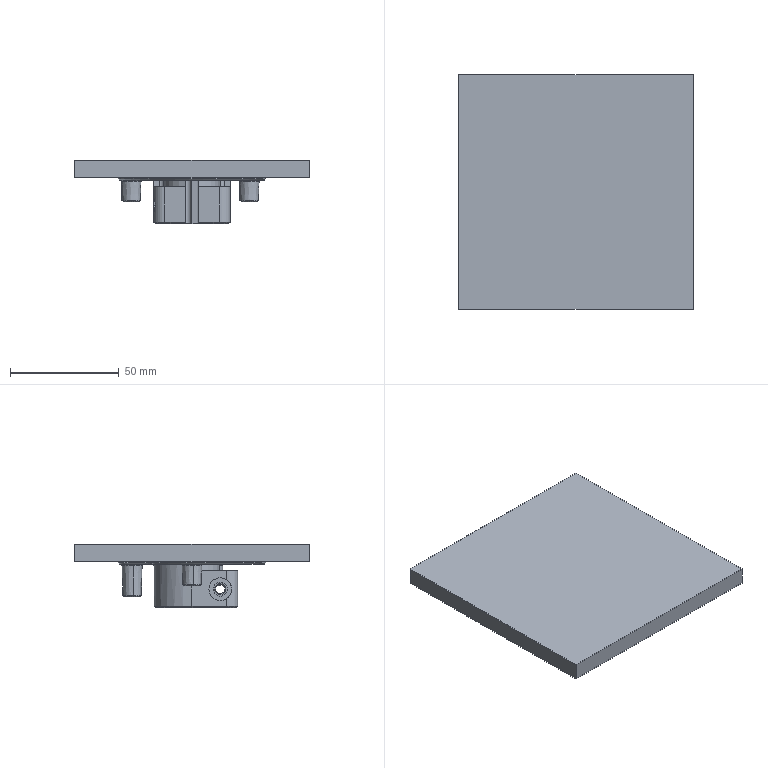NC program | NX | posted with a generic post | part box 108 x 108 x 29 mm
Whole program:
N10 G17 G21 G94 G90
(CAVITY_MILL_COPY_1 , TOOL : D6JING)
N12 T16 M6
N14 G54
N16 G17 G0 G90 X-6.712 Y-4.685 S9500 M3
N18 G43 Z30. H16
N20 Z1.5
N22 G94 G1 X-7.557 Y-4.191 Z1.449 F1000.
N24 X-8.648 Y-3.421 Z1.379
N26 X-8.373 Y-4.116 Z1.34
N28 X-8.272 Y-4.316 Z1.328
N30 X-7.476 Y-5.582 Z1.249
N32 X-6.18 Y-6.99 Z1.149
N34 X-4.625 Y-8.103 Z1.049
N36 X-2.875 Y-8.876 Z0.949
N38 X-1.004 Y-9.276 Z0.848
N40 X-0.257 Y-9.296 Z0.809
N42 X-1.353 Y-8.535 Z0.739
N44 X-3.259 Y-6.951 Z0.609
N46 X-4.208 Y-6.012 Z0.539
N48 X-5.416 Y-5.442 Z0.469
N50 X-7.557 Y-4.191 Z0.339
N52 X-8.648 Y-3.421 Z0.27
N54 X-8.373 Y-4.116 Z0.23
N56 X-8.272 Y-4.316 Z0.219
N58 X-7.476 Y-5.582 Z0.14
N60 X-6.18 Y-6.99 Z0.04
N62 X-4.625 Y-8.103 Z-0.06
N64 X-2.875 Y-8.876 Z-0.161
N66 X-1.004 Y-9.276 Z-0.261
N68 X-0.257 Y-9.296 Z-0.3
N70 G2 X-4.208 Y-6.012 R29.7 F2500.
N72 X-8.648 Y-3.421 R29.7
N74 G3 X-0.257 Y-9.296 R9.3
N76 G1 X1.796 Y-6.339
N78 G2 X-2.11 Y-3.015 R26.1
N80 X-12.018 Y4.689 R26.1
N82 G3 X8.517 Y-9.689 R12.9
N84 G2 X1.796 Y-6.339 R26.1
N86 G1 X3.849 Y-3.382
N88 G2 X0.001 Y-0.001 R22.5
N90 X-11.935 Y11.393 R22.5
N92 G3 X14.788 Y-7.318 R-16.5
N94 G2 X3.849 Y-3.382 R22.5
N96 G1 X5.902 Y-0.424
N98 G2 X2.669 Y2.416 R18.9
N100 G3 X1.358 Y3.334 R3.6
N102 G2 X-10.094 Y17.382 R18.9
N104 G3 X19.786 Y-3.541 R-20.1
N106 G2 X5.902 Y-0.424 R18.9
N108 G1 X7.954 Y2.533
N110 G2 X5.338 Y4.832 R15.3
N112 G3 X2.716 Y6.668 R7.2
N114 G2 X-6.695 Y22.735 R15.3
N116 G3 X23.653 Y1.485 R-23.7
N118 G2 X7.954 Y2.533 R15.3
N120 G1 X10.007 Y5.491
N122 G2 X8.006 Y7.249 R11.7
N124 G3 X4.074 Y10.002 R10.8
N126 G2 X-1.287 Y27.27 R11.7
N128 G3 X26.065 Y8.118 R-27.3
N130 G2 X10.007 Y5.491 R11.7
N132 G1 X12.06 Y8.448
N134 G2 X10.674 Y9.665 R8.1
N136 G3 X5.432 Y13.336 R14.4
N138 G2 X1.852 Y25.484 R8.1
N140 G1 X5.321 Y30.438
N142 G3 X26.783 Y15.411 R-30.9
N144 G1 X23.314 Y10.456
N146 G2 X12.06 Y8.448 R8.1
N148 G3 X11.816 Y8.536 R0.5
N150 G1 Z1.2
N152 G0 X-6.712 Y-4.685
N154 G1 X-7.557 Y-4.191 Z1.149 F1000.
N156 X-8.648 Y-3.421 Z1.079
N158 X-8.373 Y-4.116 Z1.04
N160 X-8.272 Y-4.316 Z1.028
N162 X-7.476 Y-5.582 Z0.949
N164 X-6.18 Y-6.99 Z0.849
N166 X-4.625 Y-8.103 Z0.749
N168 X-2.875 Y-8.876 Z0.649
N170 X-1.004 Y-9.276 Z0.548
N172 X-0.257 Y-9.296 Z0.509
N174 X-1.353 Y-8.535 Z0.439
N176 X-3.259 Y-6.951 Z0.309
N178 X-4.208 Y-6.012 Z0.239
N180 X-5.416 Y-5.442 Z0.169
N182 X-7.557 Y-4.191 Z0.039
N184 X-8.648 Y-3.421 Z-0.03
N186 X-8.373 Y-4.116 Z-0.07
N188 X-8.272 Y-4.316 Z-0.081
N190 X-7.476 Y-5.582 Z-0.16
N192 X-6.18 Y-6.99 Z-0.26
N194 X-4.625 Y-8.103 Z-0.36
N196 X-2.875 Y-8.876 Z-0.461
N198 X-1.004 Y-9.276 Z-0.561
N200 X-0.257 Y-9.296 Z-0.6
N202 G2 X-4.208 Y-6.012 R29.7 F2500.
N204 X-8.648 Y-3.421 R29.7
N206 G3 X-0.257 Y-9.296 R9.3
N208 G1 X1.796 Y-6.339
N210 G2 X-2.11 Y-3.015 R26.1
N212 X-12.018 Y4.689 R26.1
N214 G3 X8.517 Y-9.689 R12.9
N216 G2 X1.796 Y-6.339 R26.1
N218 G1 X3.849 Y-3.382
N220 G2 X0.001 Y-0.001 R22.5
N222 X-11.935 Y11.393 R22.5
N224 G3 X14.788 Y-7.318 R-16.5
N226 G2 X3.849 Y-3.382 R22.5
N228 G1 X5.902 Y-0.424
N230 G2 X2.669 Y2.416 R18.9
N232 G3 X1.358 Y3.334 R3.6
N234 G2 X-10.094 Y17.382 R18.9
N236 G3 X19.786 Y-3.541 R-20.1
N238 G2 X5.902 Y-0.424 R18.9
N240 G1 X7.954 Y2.533
N242 G2 X5.338 Y4.832 R15.3
N244 G3 X2.716 Y6.668 R7.2
N246 G2 X-6.695 Y22.735 R15.3
N248 G3 X23.653 Y1.485 R-23.7
N250 G2 X7.954 Y2.533 R15.3
N252 G1 X10.007 Y5.491
N254 G2 X8.006 Y7.249 R11.7
N256 G3 X4.074 Y10.002 R10.8
N258 G2 X-1.287 Y27.27 R11.7
N260 G3 X26.065 Y8.118 R-27.3
N262 G2 X10.007 Y5.491 R11.7
N264 G1 X12.06 Y8.448
N266 G2 X10.674 Y9.665 R8.1
N268 G3 X5.432 Y13.336 R14.4
N270 G2 X1.852 Y25.484 R8.1
N272 G1 X5.321 Y30.438
N274 G3 X26.783 Y15.411 R-30.9
N276 G1 X23.314 Y10.456
N278 G2 X12.06 Y8.448 R8.1
N280 G3 X11.816 Y8.536 R0.5
N282 G1 Z0.9
N284 G0 X-6.712 Y-4.685
N286 G1 X-7.557 Y-4.191 Z0.849 F1000.
N288 X-8.648 Y-3.421 Z0.779
N290 X-8.373 Y-4.116 Z0.74
N292 X-8.272 Y-4.316 Z0.728
N294 X-7.476 Y-5.582 Z0.649
N296 X-6.18 Y-6.99 Z0.549
N298 X-4.625 Y-8.103 Z0.449
N300 X-2.875 Y-8.876 Z0.349
N302 X-1.004 Y-9.276 Z0.248
N304 X-0.257 Y-9.296 Z0.209
N306 X-1.353 Y-8.535 Z0.139
N308 X-3.259 Y-6.951 Z0.009
N310 X-4.208 Y-6.012 Z-0.061
N312 X-5.416 Y-5.442 Z-0.131
N314 X-7.557 Y-4.191 Z-0.261
N316 X-8.648 Y-3.421 Z-0.33
N318 X-8.373 Y-4.116 Z-0.37
N320 X-8.272 Y-4.316 Z-0.381
N322 X-7.476 Y-5.582 Z-0.46
N324 X-6.18 Y-6.99 Z-0.56
N326 X-4.625 Y-8.103 Z-0.66
N328 X-2.875 Y-8.876 Z-0.761
N330 X-1.004 Y-9.276 Z-0.861
N332 X-0.257 Y-9.296 Z-0.9
N334 G2 X-4.208 Y-6.012 R29.7 F2500.
N336 X-8.648 Y-3.421 R29.7
N338 G3 X-0.257 Y-9.296 R9.3
N340 G1 X1.796 Y-6.339
N342 G2 X-2.11 Y-3.015 R26.1
N344 X-12.018 Y4.689 R26.1
N346 G3 X8.517 Y-9.689 R12.9
N348 G2 X1.796 Y-6.339 R26.1
N350 G1 X3.849 Y-3.382
N352 G2 X0.001 Y-0.001 R22.5
N354 X-11.935 Y11.393 R22.5
N356 G3 X14.788 Y-7.318 R-16.5
N358 G2 X3.849 Y-3.382 R22.5
N360 G1 X5.902 Y-0.424
N362 G2 X2.669 Y2.416 R18.9
N364 G3 X1.358 Y3.334 R3.6
N366 G2 X-10.094 Y17.382 R18.9
N368 G3 X19.786 Y-3.541 R-20.1
N370 G2 X5.902 Y-0.424 R18.9
N372 G1 X7.954 Y2.533
N374 G2 X5.338 Y4.832 R15.3
N376 G3 X2.716 Y6.668 R7.2
N378 G2 X-6.695 Y22.735 R15.3
N380 G3 X23.653 Y1.485 R-23.7
N382 G2 X7.954 Y2.533 R15.3
N384 G1 X10.007 Y5.491
N386 G2 X8.006 Y7.249 R11.7
N388 G3 X4.074 Y10.002 R10.8
N390 G2 X-1.287 Y27.27 R11.7
N392 G3 X26.065 Y8.118 R-27.3
N394 G2 X10.007 Y5.491 R11.7
N396 G1 X12.06 Y8.448
N398 G2 X10.674 Y9.665 R8.1
N400 G3 X5.432 Y13.336 R14.4
N402 G2 X1.852 Y25.484 R8.1
N404 G1 X5.321 Y30.438
N406 G3 X26.783 Y15.411 R-30.9
N408 G1 X23.314 Y10.456
N410 G2 X12.06 Y8.448 R8.1
N412 G3 X11.816 Y8.536 R0.5
N414 G1 Z0.6
N416 G0 X-6.712 Y-4.685
N418 G1 X-7.557 Y-4.191 Z0.549 F1000.
N420 X-8.648 Y-3.421 Z0.479
N422 X-8.373 Y-4.116 Z0.44
N424 X-8.272 Y-4.316 Z0.428
N426 X-7.476 Y-5.582 Z0.349
N428 X-6.18 Y-6.99 Z0.249
N430 X-4.625 Y-8.103 Z0.149
N432 X-2.875 Y-8.876 Z0.049
N434 X-1.004 Y-9.276 Z-0.052
N436 X-0.257 Y-9.296 Z-0.091
N438 X-1.353 Y-8.535 Z-0.161
N440 X-3.259 Y-6.951 Z-0.291
N442 X-4.208 Y-6.012 Z-0.361
N444 X-5.416 Y-5.442 Z-0.431
N446 X-7.557 Y-4.191 Z-0.561
N448 X-8.648 Y-3.421 Z-0.63
N450 X-8.373 Y-4.116 Z-0.67
N452 X-8.272 Y-4.316 Z-0.681
N454 X-7.476 Y-5.582 Z-0.76
N456 X-6.18 Y-6.99 Z-0.86
N458 X-4.625 Y-8.103 Z-0.96
N460 X-2.875 Y-8.876 Z-1.061
N462 X-1.004 Y-9.276 Z-1.161
N464 X-0.257 Y-9.296 Z-1.2
N466 G2 X-4.208 Y-6.012 R29.7 F2500.
N468 X-8.648 Y-3.421 R29.7
N470 G3 X-0.257 Y-9.296 R9.3
N472 G1 X1.796 Y-6.339
N474 G2 X-2.11 Y-3.015 R26.1
N476 X-12.018 Y4.689 R26.1
N478 G3 X8.517 Y-9.689 R12.9
N480 G2 X1.796 Y-6.339 R26.1
N482 G1 X3.849 Y-3.382
N484 G2 X0.001 Y-0.001 R22.5
N486 X-11.935 Y11.393 R22.5
N488 G3 X14.788 Y-7.318 R-16.5
N490 G2 X3.849 Y-3.382 R22.5
N492 G1 X5.902 Y-0.424
N494 G2 X2.669 Y2.416 R18.9
N496 G3 X1.358 Y3.334 R3.6
N498 G2 X-10.094 Y17.382 R18.9
N500 G3 X19.786 Y-3.541 R-20.1
N502 G2 X5.902 Y-0.424 R18.9
N504 G1 X7.954 Y2.533
N506 G2 X5.338 Y4.832 R15.3
N508 G3 X2.716 Y6.668 R7.2
N510 G2 X-6.695 Y22.735 R15.3
N512 G3 X23.653 Y1.485 R-23.7
N514 G2 X7.954 Y2.533 R15.3
N516 G1 X10.007 Y5.491
N518 G2 X8.006 Y7.249 R11.7
N520 G3 X4.074 Y10.002 R10.8
N522 G2 X-1.287 Y27.27 R11.7
N524 G3 X26.065 Y8.118 R-27.3
N526 G2 X10.007 Y5.491 R11.7
N528 G1 X12.06 Y8.448
N530 G2 X10.674 Y9.665 R8.1
N532 G3 X5.432 Y13.336 R14.4
N534 G2 X1.852 Y25.484 R8.1
N536 G1 X5.321 Y30.438
N538 G3 X26.783 Y15.411 R-30.9
N540 G1 X23.314 Y10.456
N542 G2 X12.06 Y8.448 R8.1
N544 G3 X11.816 Y8.536 R0.5
N546 G1 Z0.3
N548 G0 X-6.712 Y-4.685
N550 G1 X-7.557 Y-4.191 Z0.249 F1000.
N552 X-8.648 Y-3.421 Z0.179
N554 X-8.373 Y-4.116 Z0.14
N556 X-8.272 Y-4.316 Z0.128
N558 X-7.476 Y-5.582 Z0.049
N560 X-6.18 Y-6.99 Z-0.051
N562 X-4.625 Y-8.103 Z-0.151
N564 X-2.875 Y-8.876 Z-0.251
N566 X-1.004 Y-9.276 Z-0.352
N568 X-0.257 Y-9.296 Z-0.391
N570 X-1.353 Y-8.535 Z-0.461
N572 X-3.259 Y-6.951 Z-0.591
N574 X-4.208 Y-6.012 Z-0.661
N576 X-5.416 Y-5.442 Z-0.731
N578 X-7.557 Y-4.191 Z-0.861
N580 X-8.648 Y-3.421 Z-0.93
N582 X-8.373 Y-4.116 Z-0.97
N584 X-8.272 Y-4.316 Z-0.981
N586 X-7.476 Y-5.582 Z-1.06
N588 X-6.18 Y-6.99 Z-1.16
N590 X-4.625 Y-8.103 Z-1.26
N592 X-2.875 Y-8.876 Z-1.361
N594 X-1.004 Y-9.276 Z-1.461
N596 X-0.257 Y-9.296 Z-1.5
N598 G2 X-4.208 Y-6.012 R29.7 F2500.
N600 X-8.648 Y-3.421 R29.7
N602 G3 X-0.257 Y-9.296 R9.3
N604 G1 X1.796 Y-6.339
N606 G2 X-2.11 Y-3.015 R26.1
N608 X-12.018 Y4.689 R26.1
N610 G3 X8.517 Y-9.689 R12.9
N612 G2 X1.796 Y-6.339 R26.1
N614 G1 X3.849 Y-3.382
N616 G2 X0.001 Y-0.001 R22.5
N618 X-11.935 Y11.393 R22.5
N620 G3 X14.788 Y-7.318 R-16.5
N622 G2 X3.849 Y-3.382 R22.5
N624 G1 X5.902 Y-0.424
N626 G2 X2.669 Y2.416 R18.9
N628 G3 X1.358 Y3.334 R3.6
N630 G2 X-10.094 Y17.382 R18.9
N632 G3 X19.786 Y-3.541 R-20.1
N634 G2 X5.902 Y-0.424 R18.9
N636 G1 X7.954 Y2.533
N638 G2 X5.338 Y4.832 R15.3
N640 G3 X2.716 Y6.668 R7.2
N642 G2 X-6.695 Y22.735 R15.3
N644 G3 X23.653 Y1.485 R-23.7
N646 G2 X7.954 Y2.533 R15.3
N648 G1 X10.007 Y5.491
N650 G2 X8.006 Y7.249 R11.7
N652 G3 X4.074 Y10.002 R10.8
N654 G2 X-1.287 Y27.27 R11.7
N656 G3 X26.065 Y8.118 R-27.3
N658 G2 X10.007 Y5.491 R11.7
N660 G1 X12.06 Y8.448
N662 G2 X10.674 Y9.665 R8.1
N664 G3 X5.432 Y13.336 R14.4
N666 G2 X1.852 Y25.484 R8.1
N668 G1 X5.321 Y30.438
N670 G3 X26.783 Y15.411 R-30.9
N672 G1 X23.314 Y10.456
N674 G2 X12.06 Y8.448 R8.1
N676 G3 X11.816 Y8.536 R0.5
N678 G1 Z0.
N680 G0 X-6.712 Y-4.685
N682 G1 X-7.557 Y-4.191 Z-0.051 F1000.
N684 X-8.648 Y-3.421 Z-0.121
N686 X-8.373 Y-4.116 Z-0.16
N688 X-8.272 Y-4.316 Z-0.172
N690 X-7.476 Y-5.582 Z-0.251
N692 X-6.18 Y-6.99 Z-0.351
N694 X-4.625 Y-8.103 Z-0.451
N696 X-2.875 Y-8.876 Z-0.551
N698 X-1.004 Y-9.276 Z-0.652
N700 X-0.257 Y-9.296 Z-0.691
N702 X-1.353 Y-8.535 Z-0.761
N704 X-3.259 Y-6.951 Z-0.891
N706 X-4.208 Y-6.012 Z-0.961
N708 X-5.416 Y-5.442 Z-1.031
N710 X-7.557 Y-4.191 Z-1.161
N712 X-8.648 Y-3.421 Z-1.23
N714 X-8.373 Y-4.116 Z-1.27
N716 X-8.272 Y-4.316 Z-1.281
N718 X-7.476 Y-5.582 Z-1.36
N720 X-6.18 Y-6.99 Z-1.46
N722 X-4.625 Y-8.103 Z-1.56
N724 X-2.875 Y-8.876 Z-1.661
N726 X-1.004 Y-9.276 Z-1.761
N728 X-0.257 Y-9.296 Z-1.8
N730 G2 X-4.208 Y-6.012 R29.7 F2500.
N732 X-8.648 Y-3.421 R29.7
N734 G3 X-0.257 Y-9.296 R9.3
N736 G1 X1.796 Y-6.339
N738 G2 X-2.11 Y-3.015 R26.1
N740 X-12.018 Y4.689 R26.1
N742 G3 X8.517 Y-9.689 R12.9
N744 G2 X1.796 Y-6.339 R26.1
N746 G1 X3.849 Y-3.382
N748 G2 X0.001 Y-0.001 R22.5
N750 X-11.935 Y11.393 R22.5
N752 G3 X14.788 Y-7.318 R-16.5
N754 G2 X3.849 Y-3.382 R22.5
N756 G1 X5.902 Y-0.424
N758 G2 X2.669 Y2.416 R18.9
N760 G3 X1.358 Y3.334 R3.6
N762 G2 X-10.094 Y17.382 R18.9
N764 G3 X19.786 Y-3.541 R-20.1
N766 G2 X5.902 Y-0.424 R18.9
N768 G1 X7.954 Y2.533
N770 G2 X5.338 Y4.832 R15.3
N772 G3 X2.716 Y6.668 R7.2
N774 G2 X-6.695 Y22.735 R15.3
N776 G3 X23.653 Y1.485 R-23.7
N778 G2 X7.954 Y2.533 R15.3
N780 G1 X10.007 Y5.491
N782 G2 X8.006 Y7.249 R11.7
N784 G3 X4.074 Y10.002 R10.8
N786 G2 X-1.287 Y27.27 R11.7
N788 G3 X26.065 Y8.118 R-27.3
N790 G2 X10.007 Y5.491 R11.7
N792 G1 X12.06 Y8.448
N794 G2 X10.674 Y9.665 R8.1
N796 G3 X5.432 Y13.336 R14.4
N798 G2 X1.852 Y25.484 R8.1
N800 G1 X5.321 Y30.438
N802 G3 X26.783 Y15.411 R-30.9
N804 G1 X23.314 Y10.456
N806 G2 X12.06 Y8.448 R8.1
N808 G3 X11.816 Y8.536 R0.5
N810 G1 Z-0.3
N812 G0 X-6.712 Y-4.685
N814 G1 X-7.557 Y-4.191 Z-0.351 F1000.
N816 X-8.648 Y-3.421 Z-0.421
N818 X-8.373 Y-4.116 Z-0.46
N820 X-8.272 Y-4.316 Z-0.472
N822 X-7.476 Y-5.582 Z-0.551
N824 X-6.18 Y-6.99 Z-0.651
N826 X-4.625 Y-8.103 Z-0.751
N828 X-2.875 Y-8.876 Z-0.851
N830 X-1.004 Y-9.276 Z-0.952
N832 X-0.257 Y-9.296 Z-0.991
N834 X-1.353 Y-8.535 Z-1.061
N836 X-3.259 Y-6.951 Z-1.191
N838 X-4.208 Y-6.012 Z-1.261
N840 X-5.416 Y-5.442 Z-1.331
N842 X-7.557 Y-4.191 Z-1.461
N844 X-8.648 Y-3.421 Z-1.53
N846 X-8.373 Y-4.116 Z-1.57
N848 X-8.272 Y-4.316 Z-1.581
N850 X-7.476 Y-5.582 Z-1.66
N852 X-6.18 Y-6.99 Z-1.76
N854 X-4.625 Y-8.103 Z-1.86
N856 X-2.875 Y-8.876 Z-1.961
N858 X-1.004 Y-9.276 Z-2.061
N860 X-0.257 Y-9.296 Z-2.1
N862 G2 X-4.208 Y-6.012 R29.7 F2500.
N864 X-8.648 Y-3.421 R29.7
N866 G3 X-0.257 Y-9.296 R9.3
N868 G1 X1.796 Y-6.339
N870 G2 X-2.11 Y-3.015 R26.1
N872 X-12.018 Y4.689 R26.1
N874 G3 X8.517 Y-9.689 R12.9
N876 G2 X1.796 Y-6.339 R26.1
N878 G1 X3.849 Y-3.382
N880 G2 X0.001 Y-0.001 R22.5
N882 X-11.935 Y11.393 R22.5
N884 G3 X14.788 Y-7.318 R-16.5
N886 G2 X3.849 Y-3.382 R22.5
N888 G1 X5.902 Y-0.424
N890 G2 X2.669 Y2.416 R18.9
N892 G3 X1.358 Y3.334 R3.6
N894 G2 X-10.094 Y17.382 R18.9
N896 G3 X19.786 Y-3.541 R-20.1
N898 G2 X5.902 Y-0.424 R18.9
N900 G1 X7.954 Y2.533
N902 G2 X5.338 Y4.832 R15.3
N904 G3 X2.716 Y6.668 R7.2
N906 G2 X-6.695 Y22.735 R15.3
N908 G3 X23.653 Y1.485 R-23.7
N910 G2 X7.954 Y2.533 R15.3
N912 G1 X10.007 Y5.491
N914 G2 X8.006 Y7.249 R11.7
N916 G3 X4.074 Y10.002 R10.8
N918 G2 X-1.287 Y27.27 R11.7
N920 G3 X26.065 Y8.118 R-27.3
N922 G2 X10.007 Y5.491 R11.7
N924 G1 X12.06 Y8.448
N926 G2 X10.674 Y9.665 R8.1
N928 G3 X5.432 Y13.336 R14.4
N930 G2 X1.852 Y25.484 R8.1
N932 G1 X5.321 Y30.438
N934 G3 X26.783 Y15.411 R-30.9
N936 G1 X23.314 Y10.456
N938 G2 X12.06 Y8.448 R8.1
N940 G3 X11.816 Y8.536 R0.5
N942 G1 Z-0.6
N944 G0 X-6.712 Y-4.685
N946 G1 X-7.557 Y-4.191 Z-0.651 F1000.
N948 X-8.648 Y-3.421 Z-0.721
N950 X-8.373 Y-4.116 Z-0.76
N952 X-8.272 Y-4.316 Z-0.772
N954 X-7.476 Y-5.582 Z-0.851
N956 X-6.18 Y-6.99 Z-0.951
N958 X-4.625 Y-8.103 Z-1.051
N960 X-2.875 Y-8.876 Z-1.151
N962 X-1.004 Y-9.276 Z-1.252
N964 X-0.257 Y-9.296 Z-1.291
N966 X-1.353 Y-8.535 Z-1.361
N968 X-3.259 Y-6.951 Z-1.491
N970 X-4.208 Y-6.012 Z-1.561
N972 X-5.416 Y-5.442 Z-1.631
N974 X-7.557 Y-4.191 Z-1.761
N976 X-8.648 Y-3.421 Z-1.83
N978 X-8.373 Y-4.116 Z-1.87
N980 X-8.272 Y-4.316 Z-1.881
N982 X-7.476 Y-5.582 Z-1.96
N984 X-6.18 Y-6.99 Z-2.06
N986 X-4.625 Y-8.103 Z-2.16
N988 X-2.875 Y-8.876 Z-2.261
N990 X-1.004 Y-9.276 Z-2.361
N992 X-0.257 Y-9.296 Z-2.4
N994 G2 X-4.208 Y-6.012 R29.7 F2500.
N996 X-8.648 Y-3.421 R29.7
N998 G3 X-0.257 Y-9.296 R9.3
N1000 G1 X1.796 Y-6.339
N1002 G2 X-2.11 Y-3.015 R26.1
N1004 X-12.018 Y4.689 R26.1
N1006 G3 X8.517 Y-9.689 R12.9
N1008 G2 X1.796 Y-6.339 R26.1
N1010 G1 X3.849 Y-3.382
N1012 G2 X0.001 Y-0.001 R22.5
N1014 X-11.935 Y11.393 R22.5
N1016 G3 X14.788 Y-7.318 R-16.5
N1018 G2 X3.849 Y-3.382 R22.5
N1020 G1 X5.902 Y-0.424
N1022 G2 X2.669 Y2.416 R18.9
N1024 G3 X1.358 Y3.334 R3.6
N1026 G2 X-10.094 Y17.382 R18.9
N1028 G3 X19.786 Y-3.541 R-20.1
N1030 G2 X5.902 Y-0.424 R18.9
N1032 G1 X7.954 Y2.533
N1034 G2 X5.338 Y4.832 R15.3
N1036 G3 X2.716 Y6.668 R7.2
N1038 G2 X-6.695 Y22.735 R15.3
N1040 G3 X23.653 Y1.485 R-23.7
N1042 G2 X7.954 Y2.533 R15.3
N1044 G1 X10.007 Y5.491
N1046 G2 X8.006 Y7.249 R11.7
N1048 G3 X4.074 Y10.002 R10.8
N1050 G2 X-1.287 Y27.27 R11.7
N1052 G3 X26.065 Y8.118 R-27.3
N1054 G2 X10.007 Y5.491 R11.7
N1056 G1 X12.06 Y8.448
N1058 G2 X10.674 Y9.665 R8.1
N1060 G3 X5.432 Y13.336 R14.4
N1062 G2 X1.852 Y25.484 R8.1
N1064 G1 X5.321 Y30.438
N1066 G3 X26.783 Y15.411 R-30.9
N1068 G1 X23.314 Y10.456
N1070 G2 X12.06 Y8.448 R8.1
N1072 G3 X11.816 Y8.536 R0.5
N1074 G1 Z-0.9
N1076 G0 X-6.712 Y-4.685
N1078 G1 X-7.557 Y-4.191 Z-0.951 F1000.
N1080 X-8.648 Y-3.421 Z-1.021
N1082 X-8.373 Y-4.116 Z-1.06
N1084 X-8.272 Y-4.316 Z-1.072
N1086 X-7.476 Y-5.582 Z-1.151
N1088 X-6.18 Y-6.99 Z-1.251
N1090 X-4.625 Y-8.103 Z-1.351
N1092 X-2.875 Y-8.876 Z-1.451
N1094 X-1.004 Y-9.276 Z-1.552
N1096 X-0.257 Y-9.296 Z-1.591
N1098 X-1.353 Y-8.535 Z-1.661
N1100 X-3.259 Y-6.951 Z-1.791
N1102 X-4.208 Y-6.012 Z-1.861
N1104 X-5.416 Y-5.442 Z-1.931
N1106 X-7.557 Y-4.191 Z-2.061
N1108 X-8.648 Y-3.421 Z-2.13
N1110 X-8.373 Y-4.116 Z-2.17
N1112 X-8.272 Y-4.316 Z-2.181
N1114 X-7.476 Y-5.582 Z-2.26
N1116 X-6.18 Y-6.99 Z-2.36
N1118 X-4.625 Y-8.103 Z-2.46
N1120 X-2.875 Y-8.876 Z-2.561
N1122 X-1.004 Y-9.276 Z-2.661
N1124 X-0.257 Y-9.296 Z-2.7
N1126 G2 X-4.208 Y-6.012 R29.7 F2500.
N1128 X-8.648 Y-3.421 R29.7
N1130 G3 X-0.257 Y-9.296 R9.3
N1132 G1 X1.796 Y-6.339
N1134 G2 X-2.11 Y-3.015 R26.1
N1136 X-12.018 Y4.689 R26.1
N1138 G3 X8.517 Y-9.689 R12.9
N1140 G2 X1.796 Y-6.339 R26.1
N1142 G1 X3.849 Y-3.382
N1144 G2 X0.001 Y-0.001 R22.5
N1146 X-11.935 Y11.393 R22.5
N1148 G3 X14.788 Y-7.318 R-16.5
N1150 G2 X3.849 Y-3.382 R22.5
N1152 G1 X5.902 Y-0.424
N1154 G2 X2.669 Y2.416 R18.9
N1156 G3 X1.358 Y3.334 R3.6
N1158 G2 X-10.094 Y17.382 R18.9
N1160 G3 X19.786 Y-3.541 R-20.1
N1162 G2 X5.902 Y-0.424 R18.9
N1164 G1 X7.954 Y2.533
N1166 G2 X5.338 Y4.832 R15.3
N1168 G3 X2.716 Y6.668 R7.2
N1170 G2 X-6.695 Y22.735 R15.3
N1172 G3 X23.653 Y1.485 R-23.7
N1174 G2 X7.954 Y2.533 R15.3
N1176 G1 X10.007 Y5.491
N1178 G2 X8.006 Y7.249 R11.7
N1180 G3 X4.074 Y10.002 R10.8
N1182 G2 X-1.287 Y27.27 R11.7
N1184 G3 X26.065 Y8.118 R-27.3
N1186 G2 X10.007 Y5.491 R11.7
N1188 G1 X12.06 Y8.448
N1190 G2 X10.674 Y9.665 R8.1
N1192 G3 X5.432 Y13.336 R14.4
N1194 G2 X1.852 Y25.484 R8.1
N1196 G1 X5.321 Y30.438
N1198 G3 X26.783 Y15.411 R-30.9
N1200 G1 X23.314 Y10.456
N1202 G2 X12.06 Y8.448 R8.1
N1204 G3 X11.816 Y8.536 R0.5
N1206 G1 Z-1.2
N1208 G0 X-6.712 Y-4.685
N1210 G1 X-7.557 Y-4.191 Z-1.251 F1000.
N1212 X-8.648 Y-3.421 Z-1.321
N1214 X-8.373 Y-4.116 Z-1.36
N1216 X-8.272 Y-4.316 Z-1.372
N1218 X-7.476 Y-5.582 Z-1.451
N1220 X-6.18 Y-6.99 Z-1.551
N1222 X-4.625 Y-8.103 Z-1.651
N1224 X-2.875 Y-8.876 Z-1.751
N1226 X-1.004 Y-9.276 Z-1.852
N1228 X-0.257 Y-9.296 Z-1.891
N1230 X-1.353 Y-8.535 Z-1.961
N1232 X-3.259 Y-6.951 Z-2.091
N1234 X-4.208 Y-6.012 Z-2.161
N1236 X-5.416 Y-5.442 Z-2.231
N1238 X-7.557 Y-4.191 Z-2.361
N1240 X-8.648 Y-3.421 Z-2.43
N1242 X-8.373 Y-4.116 Z-2.47
N1244 X-8.272 Y-4.316 Z-2.481
N1246 X-7.476 Y-5.582 Z-2.56
N1248 X-6.18 Y-6.99 Z-2.66
N1250 X-4.625 Y-8.103 Z-2.76
N1252 X-2.875 Y-8.876 Z-2.861
N1254 X-1.004 Y-9.276 Z-2.961
N1256 X-0.257 Y-9.296 Z-3.
N1258 G2 X-4.208 Y-6.012 R29.7 F2500.
N1260 X-8.648 Y-3.421 R29.7
N1262 G3 X-0.257 Y-9.296 R9.3
N1264 G1 X1.796 Y-6.339
N1266 G2 X-2.11 Y-3.015 R26.1
N1268 X-12.018 Y4.689 R26.1
N1270 G3 X8.517 Y-9.689 R12.9
N1272 G2 X1.796 Y-6.339 R26.1
N1274 G1 X3.849 Y-3.382
N1276 G2 X0.001 Y-0.001 R22.5
N1278 X-11.935 Y11.393 R22.5
N1280 G3 X14.788 Y-7.318 R-16.5
N1282 G2 X3.849 Y-3.382 R22.5
N1284 G1 X5.902 Y-0.424
N1286 G2 X2.669 Y2.416 R18.9
N1288 G3 X1.358 Y3.334 R3.6
N1290 G2 X-10.094 Y17.382 R18.9
N1292 G3 X19.786 Y-3.541 R-20.1
N1294 G2 X5.902 Y-0.424 R18.9
N1296 G1 X7.954 Y2.533
N1298 G2 X5.338 Y4.832 R15.3
N1300 G3 X2.716 Y6.668 R7.2
N1302 G2 X-6.695 Y22.735 R15.3
N1304 G3 X23.653 Y1.485 R-23.7
N1306 G2 X7.954 Y2.533 R15.3
N1308 G1 X10.007 Y5.491
N1310 G2 X8.006 Y7.249 R11.7
N1312 G3 X4.074 Y10.002 R10.8
N1314 G2 X-1.287 Y27.27 R11.7
N1316 G3 X26.065 Y8.118 R-27.3
N1318 G2 X10.007 Y5.491 R11.7
N1320 G1 X12.06 Y8.448
N1322 G2 X10.674 Y9.665 R8.1
N1324 G3 X5.432 Y13.336 R14.4
N1326 G2 X1.852 Y25.484 R8.1
N1328 G1 X5.321 Y30.438
N1330 G3 X26.783 Y15.411 R-30.9
N1332 G1 X23.314 Y10.456
N1334 G2 X12.06 Y8.448 R8.1
N1336 G3 X11.816 Y8.536 R0.5
N1338 G1 Z-1.5
N1340 G0 X-6.712 Y-4.685
N1342 G1 X-7.557 Y-4.191 Z-1.551 F1000.
N1344 X-8.648 Y-3.421 Z-1.621
N1346 X-8.373 Y-4.116 Z-1.66
N1348 X-8.272 Y-4.316 Z-1.672
N1350 X-7.476 Y-5.582 Z-1.751
N1352 X-6.18 Y-6.99 Z-1.851
N1354 X-4.625 Y-8.103 Z-1.951
N1356 X-2.875 Y-8.876 Z-2.051
N1358 X-1.004 Y-9.276 Z-2.152
N1360 X-0.257 Y-9.296 Z-2.191
N1362 X-1.353 Y-8.535 Z-2.261
N1364 X-3.259 Y-6.951 Z-2.391
N1366 X-4.208 Y-6.012 Z-2.461
N1368 X-5.416 Y-5.442 Z-2.531
N1370 X-7.557 Y-4.191 Z-2.661
N1372 X-8.648 Y-3.421 Z-2.73
N1374 X-8.373 Y-4.116 Z-2.77
N1376 X-8.272 Y-4.316 Z-2.781
N1378 X-7.476 Y-5.582 Z-2.86
N1380 X-6.18 Y-6.99 Z-2.96
N1382 X-4.625 Y-8.103 Z-3.06
N1384 X-2.875 Y-8.876 Z-3.161
N1386 X-1.004 Y-9.276 Z-3.261
N1388 X-0.257 Y-9.296 Z-3.3
N1390 G2 X-4.208 Y-6.012 R29.7 F2500.
N1392 X-8.648 Y-3.421 R29.7
N1394 G3 X-0.257 Y-9.296 R9.3
N1396 G1 X1.796 Y-6.339
N1398 G2 X-2.11 Y-3.015 R26.1
N1400 X-12.018 Y4.689 R26.1
N1402 G3 X8.517 Y-9.689 R12.9
N1404 G2 X1.796 Y-6.339 R26.1
N1406 G1 X3.849 Y-3.382
N1408 G2 X0.001 Y-0.001 R22.5
N1410 X-11.935 Y11.393 R22.5
N1412 G3 X14.788 Y-7.318 R-16.5
N1414 G2 X3.849 Y-3.382 R22.5
N1416 G1 X5.902 Y-0.424
N1418 G2 X2.669 Y2.416 R18.9
N1420 G3 X1.358 Y3.334 R3.6
N1422 G2 X-10.094 Y17.382 R18.9
N1424 G3 X19.786 Y-3.541 R-20.1
N1426 G2 X5.902 Y-0.424 R18.9
N1428 G1 X7.954 Y2.533
N1430 G2 X5.338 Y4.832 R15.3
N1432 G3 X2.716 Y6.668 R7.2
N1434 G2 X-6.695 Y22.735 R15.3
N1436 G3 X23.653 Y1.485 R-23.7
N1438 G2 X7.954 Y2.533 R15.3
N1440 G1 X10.007 Y5.491
N1442 G2 X8.006 Y7.249 R11.7
N1444 G3 X4.074 Y10.002 R10.8
N1446 G2 X-1.287 Y27.27 R11.7
N1448 G3 X26.065 Y8.118 R-27.3
N1450 G2 X10.007 Y5.491 R11.7
N1452 G1 X12.06 Y8.448
N1454 G2 X10.674 Y9.665 R8.1
N1456 G3 X5.432 Y13.336 R14.4
N1458 G2 X1.852 Y25.484 R8.1
N1460 G1 X5.321 Y30.438
N1462 G3 X26.783 Y15.411 R-30.9
N1464 G1 X23.314 Y10.456
N1466 G2 X12.06 Y8.448 R8.1
N1468 G3 X11.816 Y8.536 R0.5
N1470 G1 Z-1.8
N1472 G0 X-6.712 Y-4.685
N1474 G1 X-7.557 Y-4.191 Z-1.851 F1000.
N1476 X-8.648 Y-3.421 Z-1.921
N1478 X-8.373 Y-4.116 Z-1.96
N1480 X-8.272 Y-4.316 Z-1.972
N1482 X-7.476 Y-5.582 Z-2.051
N1484 X-6.18 Y-6.99 Z-2.151
N1486 X-4.625 Y-8.103 Z-2.251
N1488 X-2.875 Y-8.876 Z-2.351
N1490 X-1.004 Y-9.276 Z-2.452
N1492 X-0.257 Y-9.296 Z-2.491
N1494 X-1.353 Y-8.535 Z-2.561
N1496 X-3.259 Y-6.951 Z-2.691
N1498 X-4.208 Y-6.012 Z-2.761
N1500 X-5.416 Y-5.442 Z-2.831
N1502 X-7.557 Y-4.191 Z-2.961
N1504 X-8.648 Y-3.421 Z-3.03
N1506 X-8.373 Y-4.116 Z-3.07
N1508 X-8.272 Y-4.316 Z-3.081
N1510 X-7.476 Y-5.582 Z-3.16
N1512 X-6.18 Y-6.99 Z-3.26
N1514 X-4.625 Y-8.103 Z-3.36
N1516 X-2.875 Y-8.876 Z-3.461
N1518 X-1.004 Y-9.276 Z-3.561
N1520 X-0.257 Y-9.296 Z-3.6
N1522 G2 X-4.208 Y-6.012 R29.7 F2500.
N1524 X-8.648 Y-3.421 R29.7
N1526 G3 X-0.257 Y-9.296 R9.3
N1528 G1 X1.796 Y-6.339
N1530 G2 X-2.11 Y-3.015 R26.1
N1532 X-12.018 Y4.689 R26.1
N1534 G3 X8.517 Y-9.689 R12.9
N1536 G2 X1.796 Y-6.339 R26.1
N1538 G1 X3.849 Y-3.382
N1540 G2 X0.001 Y-0.001 R22.5
N1542 X-11.935 Y11.393 R22.5
N1544 G3 X14.788 Y-7.318 R-16.5
N1546 G2 X3.849 Y-3.382 R22.5
N1548 G1 X5.902 Y-0.424
N1550 G2 X2.669 Y2.416 R18.9
N1552 G3 X1.358 Y3.334 R3.6
N1554 G2 X-10.094 Y17.382 R18.9
N1556 G3 X19.786 Y-3.541 R-20.1
N1558 G2 X5.902 Y-0.424 R18.9
N1560 G1 X7.954 Y2.533
N1562 G2 X5.338 Y4.832 R15.3
N1564 G3 X2.716 Y6.668 R7.2
N1566 G2 X-6.695 Y22.735 R15.3
N1568 G3 X23.653 Y1.485 R-23.7
N1570 G2 X7.954 Y2.533 R15.3
N1572 G1 X10.007 Y5.491
N1574 G2 X8.006 Y7.249 R11.7
N1576 G3 X4.074 Y10.002 R10.8
N1578 G2 X-1.287 Y27.27 R11.7
N1580 G3 X26.065 Y8.118 R-27.3
N1582 G2 X10.007 Y5.491 R11.7
N1584 G1 X12.06 Y8.448
N1586 G2 X10.674 Y9.665 R8.1
N1588 G3 X5.432 Y13.336 R14.4
N1590 G2 X1.852 Y25.484 R8.1
N1592 G1 X5.321 Y30.438
N1594 G3 X26.783 Y15.411 R-30.9
N1596 G1 X23.314 Y10.456
N1598 G2 X12.06 Y8.448 R8.1
N1600 G3 X11.816 Y8.536 R0.5
N1602 G1 Z-2.1
N1604 G0 X-6.712 Y-4.685
N1606 G1 X-7.557 Y-4.191 Z-2.151 F1000.
N1608 X-8.648 Y-3.421 Z-2.221
N1610 X-8.373 Y-4.116 Z-2.26
N1612 X-8.272 Y-4.316 Z-2.272
N1614 X-7.476 Y-5.582 Z-2.351
N1616 X-6.18 Y-6.99 Z-2.451
N1618 X-4.625 Y-8.103 Z-2.551
N1620 X-2.875 Y-8.876 Z-2.651
N1622 X-1.004 Y-9.276 Z-2.752
N1624 X-0.257 Y-9.296 Z-2.791
N1626 X-1.353 Y-8.535 Z-2.861
N1628 X-3.259 Y-6.951 Z-2.991
N1630 X-4.208 Y-6.012 Z-3.061
N1632 X-5.416 Y-5.442 Z-3.131
N1634 X-7.557 Y-4.191 Z-3.261
N1636 X-8.648 Y-3.421 Z-3.33
N1638 X-8.373 Y-4.116 Z-3.37
N1640 X-8.272 Y-4.316 Z-3.381
N1642 X-7.476 Y-5.582 Z-3.46
N1644 X-6.18 Y-6.99 Z-3.56
N1646 X-4.625 Y-8.103 Z-3.66
N1648 X-2.875 Y-8.876 Z-3.761
N1650 X-1.004 Y-9.276 Z-3.861
N1652 X-0.257 Y-9.296 Z-3.9
N1654 G2 X-4.208 Y-6.012 R29.7 F2500.
N1656 X-8.648 Y-3.421 R29.7
N1658 G3 X-0.257 Y-9.296 R9.3
N1660 G1 X1.796 Y-6.339
N1662 G2 X-2.11 Y-3.015 R26.1
N1664 X-12.018 Y4.689 R26.1
N1666 G3 X8.517 Y-9.689 R12.9
N1668 G2 X1.796 Y-6.339 R26.1
N1670 G1 X3.849 Y-3.382
N1672 G2 X0.001 Y-0.001 R22.5
N1674 X-11.935 Y11.393 R22.5
N1676 G3 X14.788 Y-7.318 R-16.5
N1678 G2 X3.849 Y-3.382 R22.5
N1680 G1 X5.902 Y-0.424
N1682 G2 X2.669 Y2.416 R18.9
N1684 G3 X1.358 Y3.334 R3.6
N1686 G2 X-10.094 Y17.382 R18.9
N1688 G3 X19.786 Y-3.541 R-20.1
N1690 G2 X5.902 Y-0.424 R18.9
N1692 G1 X7.954 Y2.533
N1694 G2 X5.338 Y4.832 R15.3
N1696 G3 X2.716 Y6.668 R7.2
N1698 G2 X-6.695 Y22.735 R15.3
N1700 G3 X23.653 Y1.485 R-23.7
N1702 G2 X7.954 Y2.533 R15.3
N1704 G1 X10.007 Y5.491
N1706 G2 X8.006 Y7.249 R11.7
N1708 G3 X4.074 Y10.002 R10.8
N1710 G2 X-1.287 Y27.27 R11.7
N1712 G3 X26.065 Y8.118 R-27.3
N1714 G2 X10.007 Y5.491 R11.7
N1716 G1 X12.06 Y8.448
N1718 G2 X10.674 Y9.665 R8.1
N1720 G3 X5.432 Y13.336 R14.4
N1722 G2 X1.852 Y25.484 R8.1
N1724 G1 X5.321 Y30.438
N1726 G3 X26.783 Y15.411 R-30.9
N1728 G1 X23.314 Y10.456
N1730 G2 X12.06 Y8.448 R8.1
N1732 G3 X11.816 Y8.536 R0.5
N1734 G1 Z-2.4
N1736 G0 Z30.
(FLOOR_WALL_1_COPY_1_COPY , TOOL : D6JING)
N1738 X5.248 Y12.801
N1740 Z-2.5
N1742 G1 Z-4. F1000.
N1744 G3 X4.907 Y13.294 R0.6
N1746 X5.337 Y13.105 R8.35 F1200.
N1748 G2 X10.489 Y9.498 R14.15
N1750 G3 X23.518 Y10.313 R8.35
N1752 G1 X26.761 Y14.943
N1754 G2 X4.889 Y30.258 R-30.65
N1756 G1 X1.647 Y25.627
N1758 G3 X4.907 Y13.294 R8.35
N1760 G1 X3.363 Y10.042
N1762 G3 X3.979 Y9.771 R11.95
N1764 G2 X7.82 Y7.081 R10.55
N1766 G3 X25.966 Y7.582 R11.95
N1768 G2 X-1.756 Y26.993 R-27.05
N1770 G3 X3.363 Y10.042 R11.95
N1772 G1 X1.82 Y6.79
N1774 G3 X2.622 Y6.437 R15.55
N1776 G2 X5.152 Y4.665 R6.95
N1778 G3 X23.425 Y1.092 R15.55
N1780 G2 X-6.986 Y22.385 R-23.45
N1782 G3 X1.82 Y6.79 R15.55
N1784 G1 X0.276 Y3.538
N1786 G3 X1.264 Y3.103 R19.15
N1788 G2 X2.483 Y2.249 R3.35
N1790 G3 X19.475 Y-3.843 R19.15
N1792 G2 X-10.272 Y16.986 R-19.85
N1794 G3 X0.276 Y3.538 R19.15
N1796 G1 X-1.268 Y0.285
N1798 G3 X-0.147 Y-0.21 R22.75
N1800 X14.398 Y-7.533 R22.75
N1802 G2 X-12.003 Y10.954 R-16.25
N1804 G3 X-1.268 Y0.285 R22.75
N1806 G1 X-2.811 Y-2.967
N1808 G3 X-2.256 Y-3.222 R26.35
N1810 X8.018 Y-9.784 R26.35
N1812 G2 X-11.936 Y4.189 R12.65
N1814 G3 X-2.811 Y-2.967 R26.35
N1816 G1 X-4.355 Y-6.219
N1818 G3 X-1.128 Y-8.979 R29.95
N1820 G2 X-8.052 Y-4.131 R9.05
N1822 G3 X-4.355 Y-6.219 R29.95
N1824 X-3.757 Y-6.171 R0.6
N1826 G1 Z-2.5
N1828 X1.381 Y27.862 F8000.
N1830 Z-4. F1000.
N1832 X3.106 Y27.711
N1834 G3 X3.65 Y27.965 R0.6
N1836 G1 X5.407 Y30.474 F1200.
N1838 G3 X26.787 Y15.504 R-30.95
N1840 G1 X23.273 Y10.485
N1842 G2 X10.711 Y9.699 R8.05
N1844 G3 X5.451 Y13.383 R14.45
N1846 G2 X1.893 Y25.455 R8.05
N1848 G1 X3.65 Y27.965
N1850 G3 X3.702 Y28.562 R0.6
N1852 G1 X2.719 Y29.251
N1854 Z-2.5
N1856 G0 Z30.
N1858 M5
(11_COPY_1 , TOOL : D6A45)
N1860 T01 M6
N1862 G54
N1864 G17 G0 G90 X2.108 Y24.086 S9500 M3
N1866 G43 Z30. H1
N1868 Z2.
N1870 G94 G1 Z-1. F1000.
N1872 X3.062 Y24.002
N1874 G3 X3.606 Y24.256 R0.6
N1876 G1 X7.165 Y29.339
N1878 G3 X5.855 Y32.519 R2.041
N1880 X28.555 Y16.624 R-33.041
N1882 X25.119 Y16.767 R2.041
N1884 G1 X21.56 Y11.684
N1886 G2 X12.262 Y11.103 R5.959
N1888 G3 X6.239 Y15.32 R16.541
N1890 G2 X3.606 Y24.256 R5.959
N1892 G3 X3.658 Y24.853 R0.6
N1894 G1 X3.219 Y25.795
N1896 Z2.
N1898 G0 Z30.
N1900 M5
(刀补16 , TOOL : D6JING)
N1902 T16 M6
N1904 G54
N1906 G17 G0 G90 X1.629 Y27.858 S9500 M3
N1908 G43 Z30. H16
N1910 Z-2.5
N1912 G94 G1 Z-4. F1000.
N1914 G41 X1.726 Y27.832 D16
N1916 X3.106 Y27.711
N1918 G3 X3.65 Y27.965 R0.6
N1920 G1 X5.407 Y30.474 F1200.
N1922 G3 X26.787 Y15.504 R-30.95
N1924 G1 X23.273 Y10.485
N1926 G2 X10.711 Y9.699 R8.05
N1928 G3 X5.451 Y13.383 R14.45
N1930 G2 X1.893 Y25.455 R8.05
N1932 G1 X3.65 Y27.965
N1934 G3 X3.702 Y28.562 R0.6
N1936 G40
N1938 G1 X2.719 Y29.251
N1940 Z-2.5
N1942 G0 Z30.
N1944 M5
N1946 M2